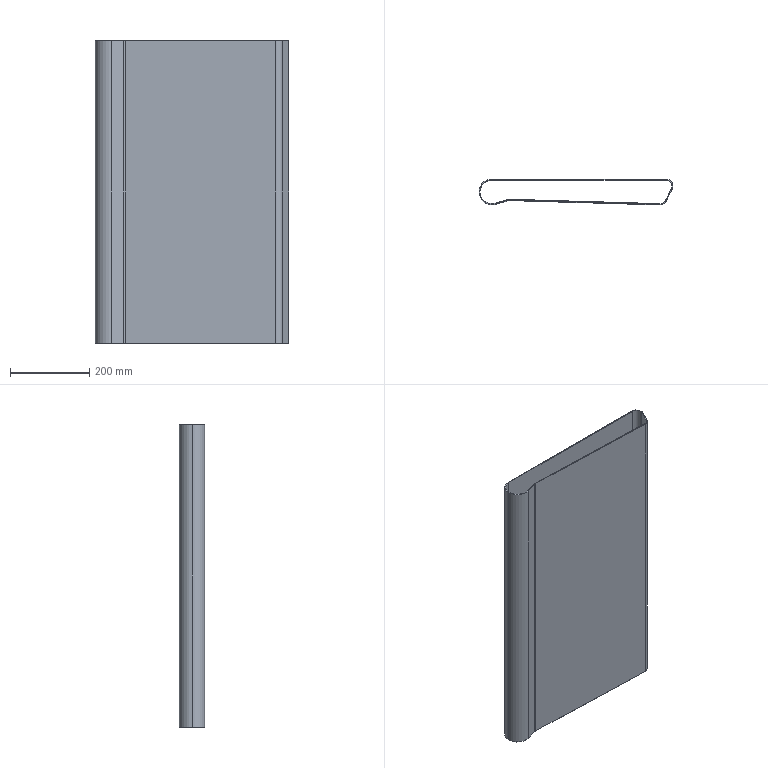Part | SolidWorks | features Extrusion 1 | 1 solid | 20 faces | box 489 x 64 x 765 mm | volume 1603169 mm3 | cylinder 10 | plane 10 | commonest cylinder face diameters 30 x2 34 x2 60 x2 64 x2 35 x1 39 x1
STEP:
#1=CARTESIAN_POINT('',(0.,30.,382.5));
#2=VERTEX_POINT('',#1);
#3=CARTESIAN_POINT('',(-30.,0.,382.5));
#4=VERTEX_POINT('',#3);
#5=CARTESIAN_POINT('',(0.,0.,382.5));
#6=DIRECTION('',(0.,0.,1.));
#7=DIRECTION('',(1.,0.,0.));
#8=AXIS2_PLACEMENT_3D('',#5,#6,#7);
#9=CIRCLE('',#8,30.);
#10=EDGE_CURVE('',#2,#4,#9,.T.);
#11=ORIENTED_EDGE('',*,*,#10,.T.);
#12=CARTESIAN_POINT('',(-30.,0.,-382.5));
#13=VERTEX_POINT('',#12);
#14=CARTESIAN_POINT('',(-30.,0.,382.5));
#15=DIRECTION('',(0.,0.,-1.));
#16=VECTOR('',#15,1000.);
#17=LINE('',#14,#16);
#18=EDGE_CURVE('',#4,#13,#17,.T.);
#19=ORIENTED_EDGE('',*,*,#18,.T.);
#20=CARTESIAN_POINT('',(0.,30.,-382.5));
#21=VERTEX_POINT('',#20);
#22=CARTESIAN_POINT('',(0.,0.,-382.5));
#23=DIRECTION('',(0.,0.,1.));
#24=DIRECTION('',(1.,0.,0.));
#25=AXIS2_PLACEMENT_3D('',#22,#23,#24);
#26=CIRCLE('',#25,30.);
#27=EDGE_CURVE('',#21,#13,#26,.T.);
#28=ORIENTED_EDGE('',*,*,#27,.F.);
#29=CARTESIAN_POINT('',(0.,30.,382.5));
#30=DIRECTION('',(0.,0.,-1.));
#31=VECTOR('',#30,1000.);
#32=LINE('',#29,#31);
#33=EDGE_CURVE('',#2,#21,#32,.T.);
#34=ORIENTED_EDGE('',*,*,#33,.F.);
#35=EDGE_LOOP('',(#11,#19,#28,#34));
#36=FACE_OUTER_BOUND('',#35,.T.);
#37=CARTESIAN_POINT('',(0.,0.,382.5));
#38=DIRECTION('',(0.,0.,-1.));
#39=DIRECTION('',(-1.,0.,0.));
#40=AXIS2_PLACEMENT_3D('',#37,#38,#39);
#41=CYLINDRICAL_SURFACE('',#40,30.);
#42=ADVANCED_FACE('',(#36),#41,.F.);
#43=CARTESIAN_POINT('',(-32.,0.,382.5));
#44=VERTEX_POINT('',#43);
#45=CARTESIAN_POINT('',(8.903,-30.737,382.5));
#46=VERTEX_POINT('',#45);
#47=CARTESIAN_POINT('',(0.,0.,382.5));
#48=DIRECTION('',(0.,0.,1.));
#49=DIRECTION('',(1.,0.,0.));
#50=AXIS2_PLACEMENT_3D('',#47,#48,#49);
#51=CIRCLE('',#50,32.);
#52=EDGE_CURVE('',#44,#46,#51,.T.);
#53=ORIENTED_EDGE('',*,*,#52,.F.);
#54=CARTESIAN_POINT('',(-32.,0.,-382.5));
#55=VERTEX_POINT('',#54);
#56=CARTESIAN_POINT('',(-32.,0.,382.5));
#57=DIRECTION('',(0.,0.,-1.));
#58=VECTOR('',#57,1000.);
#59=LINE('',#56,#58);
#60=EDGE_CURVE('',#44,#55,#59,.T.);
#61=ORIENTED_EDGE('',*,*,#60,.T.);
#62=CARTESIAN_POINT('',(8.903,-30.737,-382.5));
#63=VERTEX_POINT('',#62);
#64=CARTESIAN_POINT('',(0.,0.,-382.5));
#65=DIRECTION('',(0.,0.,1.));
#66=DIRECTION('',(1.,0.,0.));
#67=AXIS2_PLACEMENT_3D('',#64,#65,#66);
#68=CIRCLE('',#67,32.);
#69=EDGE_CURVE('',#55,#63,#68,.T.);
#70=ORIENTED_EDGE('',*,*,#69,.T.);
#71=CARTESIAN_POINT('',(8.903,-30.737,382.5));
#72=DIRECTION('',(0.,0.,-1.));
#73=VECTOR('',#72,1000.);
#74=LINE('',#71,#73);
#75=EDGE_CURVE('',#46,#63,#74,.T.);
#76=ORIENTED_EDGE('',*,*,#75,.F.);
#77=EDGE_LOOP('',(#53,#61,#70,#76));
#78=FACE_OUTER_BOUND('',#77,.T.);
#79=CARTESIAN_POINT('',(0.,0.,382.5));
#80=DIRECTION('',(0.,0.,-1.));
#81=DIRECTION('',(-1.,0.,0.));
#82=AXIS2_PLACEMENT_3D('',#79,#80,#81);
#83=CYLINDRICAL_SURFACE('',#82,32.);
#84=ADVANCED_FACE('',(#78),#83,.T.);
#85=CARTESIAN_POINT('',(0.,32.,382.5));
#86=VERTEX_POINT('',#85);
#87=CARTESIAN_POINT('',(0.,0.,382.5));
#88=DIRECTION('',(0.,0.,1.));
#89=DIRECTION('',(1.,0.,0.));
#90=AXIS2_PLACEMENT_3D('',#87,#88,#89);
#91=CIRCLE('',#90,32.);
#92=EDGE_CURVE('',#86,#44,#91,.T.);
#93=ORIENTED_EDGE('',*,*,#92,.T.);
#94=ORIENTED_EDGE('',*,*,#52,.T.);
#95=CARTESIAN_POINT('',(40.131,-21.691,382.5));
#96=VERTEX_POINT('',#95);
#97=CARTESIAN_POINT('',(8.903,-30.737,382.5));
#98=DIRECTION('',(0.9605,0.2782,0.));
#99=VECTOR('',#98,1000.);
#100=LINE('',#97,#99);
#101=EDGE_CURVE('',#46,#96,#100,.T.);
#102=ORIENTED_EDGE('',*,*,#101,.T.);
#103=CARTESIAN_POINT('',(45.507,-21.007,382.5));
#104=VERTEX_POINT('',#103);
#105=CARTESIAN_POINT('',(45.,-38.5,382.5));
#106=DIRECTION('',(0.,0.,-1.));
#107=DIRECTION('',(1.,0.,0.));
#108=AXIS2_PLACEMENT_3D('',#105,#106,#107);
#109=CIRCLE('',#108,17.5);
#110=EDGE_CURVE('',#96,#104,#109,.T.);
#111=ORIENTED_EDGE('',*,*,#110,.T.);
#112=CARTESIAN_POINT('',(424.507,-31.993,382.5));
#113=VERTEX_POINT('',#112);
#114=CARTESIAN_POINT('',(45.507,-21.007,382.5));
#115=DIRECTION('',(0.9996,-0.02897,0.));
#116=VECTOR('',#115,1000.);
#117=LINE('',#114,#116);
#118=EDGE_CURVE('',#104,#113,#117,.T.);
#119=ORIENTED_EDGE('',*,*,#118,.T.);
#120=CARTESIAN_POINT('',(440.205,-22.603,382.5));
#121=VERTEX_POINT('',#120);
#122=CARTESIAN_POINT('',(425.,-15.,382.5));
#123=DIRECTION('',(0.,0.,1.));
#124=DIRECTION('',(1.,0.,0.));
#125=AXIS2_PLACEMENT_3D('',#122,#123,#124);
#126=CIRCLE('',#125,17.);
#127=EDGE_CURVE('',#113,#121,#126,.T.);
#128=ORIENTED_EDGE('',*,*,#127,.T.);
#129=CARTESIAN_POINT('',(455.205,7.397,382.5));
#130=VERTEX_POINT('',#129);
#131=CARTESIAN_POINT('',(455.205,7.397,382.5));
#132=DIRECTION('',(0.4472,0.8944,0.));
#133=VECTOR('',#132,1000.);
#134=LINE('',#131,#133);
#135=EDGE_CURVE('',#121,#130,#134,.T.);
#136=ORIENTED_EDGE('',*,*,#135,.T.);
#137=CARTESIAN_POINT('',(440.,32.,382.5));
#138=VERTEX_POINT('',#137);
#139=CARTESIAN_POINT('',(440.,15.,382.5));
#140=DIRECTION('',(0.,0.,1.));
#141=DIRECTION('',(1.,0.,0.));
#142=AXIS2_PLACEMENT_3D('',#139,#140,#141);
#143=CIRCLE('',#142,17.);
#144=EDGE_CURVE('',#130,#138,#143,.T.);
#145=ORIENTED_EDGE('',*,*,#144,.T.);
#146=CARTESIAN_POINT('',(0.,32.,382.5));
#147=DIRECTION('',(-1.,0.,0.));
#148=VECTOR('',#147,1000.);
#149=LINE('',#146,#148);
#150=EDGE_CURVE('',#138,#86,#149,.T.);
#151=ORIENTED_EDGE('',*,*,#150,.T.);
#152=EDGE_LOOP('',(#93,#94,#102,#111,#119,#128,#136,#145,#151));
#153=FACE_OUTER_BOUND('',#152,.T.);
#154=CARTESIAN_POINT('',(8.347,-28.815,382.5));
#155=VERTEX_POINT('',#154);
#156=CARTESIAN_POINT('',(39.575,-19.77,382.5));
#157=VERTEX_POINT('',#156);
#158=CARTESIAN_POINT('',(8.347,-28.815,382.5));
#159=DIRECTION('',(0.9605,0.2782,0.));
#160=VECTOR('',#159,1000.);
#161=LINE('',#158,#160);
#162=EDGE_CURVE('',#155,#157,#161,.T.);
#163=ORIENTED_EDGE('',*,*,#162,.F.);
#164=CARTESIAN_POINT('',(0.,0.,382.5));
#165=DIRECTION('',(0.,0.,1.));
#166=DIRECTION('',(1.,0.,0.));
#167=AXIS2_PLACEMENT_3D('',#164,#165,#166);
#168=CIRCLE('',#167,30.);
#169=EDGE_CURVE('',#4,#155,#168,.T.);
#170=ORIENTED_EDGE('',*,*,#169,.F.);
#171=ORIENTED_EDGE('',*,*,#10,.F.);
#172=CARTESIAN_POINT('',(440.,30.,382.5));
#173=VERTEX_POINT('',#172);
#174=CARTESIAN_POINT('',(0.,30.,382.5));
#175=DIRECTION('',(-1.,0.,0.));
#176=VECTOR('',#175,1000.);
#177=LINE('',#174,#176);
#178=EDGE_CURVE('',#173,#2,#177,.T.);
#179=ORIENTED_EDGE('',*,*,#178,.F.);
#180=CARTESIAN_POINT('',(453.416,8.292,382.5));
#181=VERTEX_POINT('',#180);
#182=CARTESIAN_POINT('',(440.,15.,382.5));
#183=DIRECTION('',(0.,0.,1.));
#184=DIRECTION('',(1.,0.,0.));
#185=AXIS2_PLACEMENT_3D('',#182,#183,#184);
#186=CIRCLE('',#185,15.);
#187=EDGE_CURVE('',#181,#173,#186,.T.);
#188=ORIENTED_EDGE('',*,*,#187,.F.);
#189=CARTESIAN_POINT('',(438.416,-21.708,382.5));
#190=VERTEX_POINT('',#189);
#191=CARTESIAN_POINT('',(453.416,8.292,382.5));
#192=DIRECTION('',(0.4472,0.8944,0.));
#193=VECTOR('',#192,1000.);
#194=LINE('',#191,#193);
#195=EDGE_CURVE('',#190,#181,#194,.T.);
#196=ORIENTED_EDGE('',*,*,#195,.F.);
#197=CARTESIAN_POINT('',(424.565,-29.994,382.5));
#198=VERTEX_POINT('',#197);
#199=CARTESIAN_POINT('',(425.,-15.,382.5));
#200=DIRECTION('',(0.,0.,1.));
#201=DIRECTION('',(1.,0.,0.));
#202=AXIS2_PLACEMENT_3D('',#199,#200,#201);
#203=CIRCLE('',#202,15.);
#204=EDGE_CURVE('',#198,#190,#203,.T.);
#205=ORIENTED_EDGE('',*,*,#204,.F.);
#206=CARTESIAN_POINT('',(45.565,-19.008,382.5));
#207=VERTEX_POINT('',#206);
#208=CARTESIAN_POINT('',(45.565,-19.008,382.5));
#209=DIRECTION('',(0.9996,-0.02897,0.));
#210=VECTOR('',#209,1000.);
#211=LINE('',#208,#210);
#212=EDGE_CURVE('',#207,#198,#211,.T.);
#213=ORIENTED_EDGE('',*,*,#212,.F.);
#214=CARTESIAN_POINT('',(45.,-38.5,382.5));
#215=DIRECTION('',(0.,0.,-1.));
#216=DIRECTION('',(1.,0.,0.));
#217=AXIS2_PLACEMENT_3D('',#214,#215,#216);
#218=CIRCLE('',#217,19.5);
#219=EDGE_CURVE('',#157,#207,#218,.T.);
#220=ORIENTED_EDGE('',*,*,#219,.F.);
#221=EDGE_LOOP('',(#163,#170,#171,#179,#188,#196,#205,#213,#220));
#222=FACE_BOUND('',#221,.T.);
#223=CARTESIAN_POINT('',(0.,0.,382.5));
#224=DIRECTION('',(0.,0.,1.));
#225=DIRECTION('',(1.,0.,0.));
#226=AXIS2_PLACEMENT_3D('',#223,#224,#225);
#227=PLANE('',#226);
#228=ADVANCED_FACE('',(#153,#222),#227,.T.);
#229=CARTESIAN_POINT('',(0.,32.,-382.5));
#230=VERTEX_POINT('',#229);
#231=CARTESIAN_POINT('',(0.,0.,-382.5));
#232=DIRECTION('',(0.,0.,1.));
#233=DIRECTION('',(1.,0.,0.));
#234=AXIS2_PLACEMENT_3D('',#231,#232,#233);
#235=CIRCLE('',#234,32.);
#236=EDGE_CURVE('',#230,#55,#235,.T.);
#237=ORIENTED_EDGE('',*,*,#236,.F.);
#238=CARTESIAN_POINT('',(440.,32.,-382.5));
#239=VERTEX_POINT('',#238);
#240=CARTESIAN_POINT('',(0.,32.,-382.5));
#241=DIRECTION('',(-1.,0.,0.));
#242=VECTOR('',#241,1000.);
#243=LINE('',#240,#242);
#244=EDGE_CURVE('',#239,#230,#243,.T.);
#245=ORIENTED_EDGE('',*,*,#244,.F.);
#246=CARTESIAN_POINT('',(455.205,7.397,-382.5));
#247=VERTEX_POINT('',#246);
#248=CARTESIAN_POINT('',(440.,15.,-382.5));
#249=DIRECTION('',(0.,0.,1.));
#250=DIRECTION('',(1.,0.,0.));
#251=AXIS2_PLACEMENT_3D('',#248,#249,#250);
#252=CIRCLE('',#251,17.);
#253=EDGE_CURVE('',#247,#239,#252,.T.);
#254=ORIENTED_EDGE('',*,*,#253,.F.);
#255=CARTESIAN_POINT('',(440.205,-22.603,-382.5));
#256=VERTEX_POINT('',#255);
#257=CARTESIAN_POINT('',(455.205,7.397,-382.5));
#258=DIRECTION('',(0.4472,0.8944,0.));
#259=VECTOR('',#258,1000.);
#260=LINE('',#257,#259);
#261=EDGE_CURVE('',#256,#247,#260,.T.);
#262=ORIENTED_EDGE('',*,*,#261,.F.);
#263=CARTESIAN_POINT('',(424.507,-31.993,-382.5));
#264=VERTEX_POINT('',#263);
#265=CARTESIAN_POINT('',(425.,-15.,-382.5));
#266=DIRECTION('',(0.,0.,1.));
#267=DIRECTION('',(1.,0.,0.));
#268=AXIS2_PLACEMENT_3D('',#265,#266,#267);
#269=CIRCLE('',#268,17.);
#270=EDGE_CURVE('',#264,#256,#269,.T.);
#271=ORIENTED_EDGE('',*,*,#270,.F.);
#272=CARTESIAN_POINT('',(45.507,-21.007,-382.5));
#273=VERTEX_POINT('',#272);
#274=CARTESIAN_POINT('',(45.507,-21.007,-382.5));
#275=DIRECTION('',(0.9996,-0.02897,0.));
#276=VECTOR('',#275,1000.);
#277=LINE('',#274,#276);
#278=EDGE_CURVE('',#273,#264,#277,.T.);
#279=ORIENTED_EDGE('',*,*,#278,.F.);
#280=CARTESIAN_POINT('',(40.131,-21.691,-382.5));
#281=VERTEX_POINT('',#280);
#282=CARTESIAN_POINT('',(45.,-38.5,-382.5));
#283=DIRECTION('',(0.,0.,-1.));
#284=DIRECTION('',(1.,0.,0.));
#285=AXIS2_PLACEMENT_3D('',#282,#283,#284);
#286=CIRCLE('',#285,17.5);
#287=EDGE_CURVE('',#281,#273,#286,.T.);
#288=ORIENTED_EDGE('',*,*,#287,.F.);
#289=CARTESIAN_POINT('',(8.903,-30.737,-382.5));
#290=DIRECTION('',(0.9605,0.2782,0.));
#291=VECTOR('',#290,1000.);
#292=LINE('',#289,#291);
#293=EDGE_CURVE('',#63,#281,#292,.T.);
#294=ORIENTED_EDGE('',*,*,#293,.F.);
#295=ORIENTED_EDGE('',*,*,#69,.F.);
#296=EDGE_LOOP('',(#237,#245,#254,#262,#271,#279,#288,#294,#295));
#297=FACE_OUTER_BOUND('',#296,.T.);
#298=ORIENTED_EDGE('',*,*,#27,.T.);
#299=CARTESIAN_POINT('',(8.347,-28.815,-382.5));
#300=VERTEX_POINT('',#299);
#301=CARTESIAN_POINT('',(0.,0.,-382.5));
#302=DIRECTION('',(0.,0.,1.));
#303=DIRECTION('',(1.,0.,0.));
#304=AXIS2_PLACEMENT_3D('',#301,#302,#303);
#305=CIRCLE('',#304,30.);
#306=EDGE_CURVE('',#13,#300,#305,.T.);
#307=ORIENTED_EDGE('',*,*,#306,.T.);
#308=CARTESIAN_POINT('',(39.575,-19.77,-382.5));
#309=VERTEX_POINT('',#308);
#310=CARTESIAN_POINT('',(8.347,-28.815,-382.5));
#311=DIRECTION('',(0.9605,0.2782,0.));
#312=VECTOR('',#311,1000.);
#313=LINE('',#310,#312);
#314=EDGE_CURVE('',#300,#309,#313,.T.);
#315=ORIENTED_EDGE('',*,*,#314,.T.);
#316=CARTESIAN_POINT('',(45.565,-19.008,-382.5));
#317=VERTEX_POINT('',#316);
#318=CARTESIAN_POINT('',(45.,-38.5,-382.5));
#319=DIRECTION('',(0.,0.,-1.));
#320=DIRECTION('',(1.,0.,0.));
#321=AXIS2_PLACEMENT_3D('',#318,#319,#320);
#322=CIRCLE('',#321,19.5);
#323=EDGE_CURVE('',#309,#317,#322,.T.);
#324=ORIENTED_EDGE('',*,*,#323,.T.);
#325=CARTESIAN_POINT('',(424.565,-29.994,-382.5));
#326=VERTEX_POINT('',#325);
#327=CARTESIAN_POINT('',(45.565,-19.008,-382.5));
#328=DIRECTION('',(0.9996,-0.02897,0.));
#329=VECTOR('',#328,1000.);
#330=LINE('',#327,#329);
#331=EDGE_CURVE('',#317,#326,#330,.T.);
#332=ORIENTED_EDGE('',*,*,#331,.T.);
#333=CARTESIAN_POINT('',(438.416,-21.708,-382.5));
#334=VERTEX_POINT('',#333);
#335=CARTESIAN_POINT('',(425.,-15.,-382.5));
#336=DIRECTION('',(0.,0.,1.));
#337=DIRECTION('',(1.,0.,0.));
#338=AXIS2_PLACEMENT_3D('',#335,#336,#337);
#339=CIRCLE('',#338,15.);
#340=EDGE_CURVE('',#326,#334,#339,.T.);
#341=ORIENTED_EDGE('',*,*,#340,.T.);
#342=CARTESIAN_POINT('',(453.416,8.292,-382.5));
#343=VERTEX_POINT('',#342);
#344=CARTESIAN_POINT('',(453.416,8.292,-382.5));
#345=DIRECTION('',(0.4472,0.8944,0.));
#346=VECTOR('',#345,1000.);
#347=LINE('',#344,#346);
#348=EDGE_CURVE('',#334,#343,#347,.T.);
#349=ORIENTED_EDGE('',*,*,#348,.T.);
#350=CARTESIAN_POINT('',(440.,30.,-382.5));
#351=VERTEX_POINT('',#350);
#352=CARTESIAN_POINT('',(440.,15.,-382.5));
#353=DIRECTION('',(0.,0.,1.));
#354=DIRECTION('',(1.,0.,0.));
#355=AXIS2_PLACEMENT_3D('',#352,#353,#354);
#356=CIRCLE('',#355,15.);
#357=EDGE_CURVE('',#343,#351,#356,.T.);
#358=ORIENTED_EDGE('',*,*,#357,.T.);
#359=CARTESIAN_POINT('',(0.,30.,-382.5));
#360=DIRECTION('',(-1.,0.,0.));
#361=VECTOR('',#360,1000.);
#362=LINE('',#359,#361);
#363=EDGE_CURVE('',#351,#21,#362,.T.);
#364=ORIENTED_EDGE('',*,*,#363,.T.);
#365=EDGE_LOOP('',(#298,#307,#315,#324,#332,#341,#349,#358,#364));
#366=FACE_BOUND('',#365,.T.);
#367=CARTESIAN_POINT('',(0.,0.,-382.5));
#368=DIRECTION('',(0.,0.,1.));
#369=DIRECTION('',(1.,0.,0.));
#370=AXIS2_PLACEMENT_3D('',#367,#368,#369);
#371=PLANE('',#370);
#372=ADVANCED_FACE('',(#297,#366),#371,.F.);
#373=ORIENTED_EDGE('',*,*,#60,.F.);
#374=ORIENTED_EDGE('',*,*,#92,.F.);
#375=CARTESIAN_POINT('',(0.,32.,382.5));
#376=DIRECTION('',(0.,0.,-1.));
#377=VECTOR('',#376,1000.);
#378=LINE('',#375,#377);
#379=EDGE_CURVE('',#86,#230,#378,.T.);
#380=ORIENTED_EDGE('',*,*,#379,.T.);
#381=ORIENTED_EDGE('',*,*,#236,.T.);
#382=EDGE_LOOP('',(#373,#374,#380,#381));
#383=FACE_OUTER_BOUND('',#382,.T.);
#384=CARTESIAN_POINT('',(0.,0.,382.5));
#385=DIRECTION('',(0.,0.,-1.));
#386=DIRECTION('',(-1.,0.,0.));
#387=AXIS2_PLACEMENT_3D('',#384,#385,#386);
#388=CYLINDRICAL_SURFACE('',#387,32.);
#389=ADVANCED_FACE('',(#383),#388,.T.);
#390=ORIENTED_EDGE('',*,*,#293,.T.);
#391=CARTESIAN_POINT('',(40.131,-21.691,382.5));
#392=DIRECTION('',(0.,0.,-1.));
#393=VECTOR('',#392,1000.);
#394=LINE('',#391,#393);
#395=EDGE_CURVE('',#96,#281,#394,.T.);
#396=ORIENTED_EDGE('',*,*,#395,.F.);
#397=ORIENTED_EDGE('',*,*,#101,.F.);
#398=ORIENTED_EDGE('',*,*,#75,.T.);
#399=EDGE_LOOP('',(#390,#396,#397,#398));
#400=FACE_OUTER_BOUND('',#399,.T.);
#401=CARTESIAN_POINT('',(8.903,-30.737,382.5));
#402=DIRECTION('',(-0.2782,0.9605,0.));
#403=DIRECTION('',(-0.9605,-0.2782,0.));
#404=AXIS2_PLACEMENT_3D('',#401,#402,#403);
#405=PLANE('',#404);
#406=ADVANCED_FACE('',(#400),#405,.F.);
#407=ORIENTED_EDGE('',*,*,#287,.T.);
#408=CARTESIAN_POINT('',(45.507,-21.007,382.5));
#409=DIRECTION('',(0.,0.,-1.));
#410=VECTOR('',#409,1000.);
#411=LINE('',#408,#410);
#412=EDGE_CURVE('',#104,#273,#411,.T.);
#413=ORIENTED_EDGE('',*,*,#412,.F.);
#414=ORIENTED_EDGE('',*,*,#110,.F.);
#415=ORIENTED_EDGE('',*,*,#395,.T.);
#416=EDGE_LOOP('',(#407,#413,#414,#415));
#417=FACE_OUTER_BOUND('',#416,.T.);
#418=CARTESIAN_POINT('',(45.,-38.5,382.5));
#419=DIRECTION('',(0.,0.,-1.));
#420=DIRECTION('',(-1.,0.,0.));
#421=AXIS2_PLACEMENT_3D('',#418,#419,#420);
#422=CYLINDRICAL_SURFACE('',#421,17.5);
#423=ADVANCED_FACE('',(#417),#422,.F.);
#424=ORIENTED_EDGE('',*,*,#278,.T.);
#425=CARTESIAN_POINT('',(424.507,-31.993,382.5));
#426=DIRECTION('',(0.,0.,-1.));
#427=VECTOR('',#426,1000.);
#428=LINE('',#425,#427);
#429=EDGE_CURVE('',#113,#264,#428,.T.);
#430=ORIENTED_EDGE('',*,*,#429,.F.);
#431=ORIENTED_EDGE('',*,*,#118,.F.);
#432=ORIENTED_EDGE('',*,*,#412,.T.);
#433=EDGE_LOOP('',(#424,#430,#431,#432));
#434=FACE_OUTER_BOUND('',#433,.T.);
#435=CARTESIAN_POINT('',(45.507,-21.007,382.5));
#436=DIRECTION('',(0.02897,0.9996,0.));
#437=DIRECTION('',(-0.9996,0.02897,0.));
#438=AXIS2_PLACEMENT_3D('',#435,#436,#437);
#439=PLANE('',#438);
#440=ADVANCED_FACE('',(#434),#439,.F.);
#441=ORIENTED_EDGE('',*,*,#270,.T.);
#442=CARTESIAN_POINT('',(440.205,-22.603,382.5));
#443=DIRECTION('',(0.,0.,-1.));
#444=VECTOR('',#443,1000.);
#445=LINE('',#442,#444);
#446=EDGE_CURVE('',#121,#256,#445,.T.);
#447=ORIENTED_EDGE('',*,*,#446,.F.);
#448=ORIENTED_EDGE('',*,*,#127,.F.);
#449=ORIENTED_EDGE('',*,*,#429,.T.);
#450=EDGE_LOOP('',(#441,#447,#448,#449));
#451=FACE_OUTER_BOUND('',#450,.T.);
#452=CARTESIAN_POINT('',(425.,-15.,382.5));
#453=DIRECTION('',(0.,0.,-1.));
#454=DIRECTION('',(-1.,0.,0.));
#455=AXIS2_PLACEMENT_3D('',#452,#453,#454);
#456=CYLINDRICAL_SURFACE('',#455,17.);
#457=ADVANCED_FACE('',(#451),#456,.T.);
#458=ORIENTED_EDGE('',*,*,#261,.T.);
#459=CARTESIAN_POINT('',(455.205,7.397,382.5));
#460=DIRECTION('',(0.,0.,-1.));
#461=VECTOR('',#460,1000.);
#462=LINE('',#459,#461);
#463=EDGE_CURVE('',#130,#247,#462,.T.);
#464=ORIENTED_EDGE('',*,*,#463,.F.);
#465=ORIENTED_EDGE('',*,*,#135,.F.);
#466=ORIENTED_EDGE('',*,*,#446,.T.);
#467=EDGE_LOOP('',(#458,#464,#465,#466));
#468=FACE_OUTER_BOUND('',#467,.T.);
#469=CARTESIAN_POINT('',(455.205,7.397,382.5));
#470=DIRECTION('',(-0.8944,0.4472,0.));
#471=DIRECTION('',(-0.4472,-0.8944,0.));
#472=AXIS2_PLACEMENT_3D('',#469,#470,#471);
#473=PLANE('',#472);
#474=ADVANCED_FACE('',(#468),#473,.F.);
#475=ORIENTED_EDGE('',*,*,#253,.T.);
#476=CARTESIAN_POINT('',(440.,32.,382.5));
#477=DIRECTION('',(0.,0.,-1.));
#478=VECTOR('',#477,1000.);
#479=LINE('',#476,#478);
#480=EDGE_CURVE('',#138,#239,#479,.T.);
#481=ORIENTED_EDGE('',*,*,#480,.F.);
#482=ORIENTED_EDGE('',*,*,#144,.F.);
#483=ORIENTED_EDGE('',*,*,#463,.T.);
#484=EDGE_LOOP('',(#475,#481,#482,#483));
#485=FACE_OUTER_BOUND('',#484,.T.);
#486=CARTESIAN_POINT('',(440.,15.,382.5));
#487=DIRECTION('',(0.,0.,-1.));
#488=DIRECTION('',(-1.,0.,0.));
#489=AXIS2_PLACEMENT_3D('',#486,#487,#488);
#490=CYLINDRICAL_SURFACE('',#489,17.);
#491=ADVANCED_FACE('',(#485),#490,.T.);
#492=ORIENTED_EDGE('',*,*,#244,.T.);
#493=ORIENTED_EDGE('',*,*,#379,.F.);
#494=ORIENTED_EDGE('',*,*,#150,.F.);
#495=ORIENTED_EDGE('',*,*,#480,.T.);
#496=EDGE_LOOP('',(#492,#493,#494,#495));
#497=FACE_OUTER_BOUND('',#496,.T.);
#498=CARTESIAN_POINT('',(0.,32.,382.5));
#499=DIRECTION('',(0.,-1.,0.));
#500=DIRECTION('',(1.,0.,0.));
#501=AXIS2_PLACEMENT_3D('',#498,#499,#500);
#502=PLANE('',#501);
#503=ADVANCED_FACE('',(#497),#502,.F.);
#504=ORIENTED_EDGE('',*,*,#18,.F.);
#505=ORIENTED_EDGE('',*,*,#169,.T.);
#506=CARTESIAN_POINT('',(8.347,-28.815,382.5));
#507=DIRECTION('',(0.,0.,-1.));
#508=VECTOR('',#507,1000.);
#509=LINE('',#506,#508);
#510=EDGE_CURVE('',#155,#300,#509,.T.);
#511=ORIENTED_EDGE('',*,*,#510,.T.);
#512=ORIENTED_EDGE('',*,*,#306,.F.);
#513=EDGE_LOOP('',(#504,#505,#511,#512));
#514=FACE_OUTER_BOUND('',#513,.T.);
#515=CARTESIAN_POINT('',(0.,0.,382.5));
#516=DIRECTION('',(0.,0.,-1.));
#517=DIRECTION('',(-1.,0.,0.));
#518=AXIS2_PLACEMENT_3D('',#515,#516,#517);
#519=CYLINDRICAL_SURFACE('',#518,30.);
#520=ADVANCED_FACE('',(#514),#519,.F.);
#521=ORIENTED_EDGE('',*,*,#314,.F.);
#522=ORIENTED_EDGE('',*,*,#510,.F.);
#523=ORIENTED_EDGE('',*,*,#162,.T.);
#524=CARTESIAN_POINT('',(39.575,-19.77,382.5));
#525=DIRECTION('',(0.,0.,-1.));
#526=VECTOR('',#525,1000.);
#527=LINE('',#524,#526);
#528=EDGE_CURVE('',#157,#309,#527,.T.);
#529=ORIENTED_EDGE('',*,*,#528,.T.);
#530=EDGE_LOOP('',(#521,#522,#523,#529));
#531=FACE_OUTER_BOUND('',#530,.T.);
#532=CARTESIAN_POINT('',(8.347,-28.815,382.5));
#533=DIRECTION('',(-0.2782,0.9605,0.));
#534=DIRECTION('',(-0.9605,-0.2782,0.));
#535=AXIS2_PLACEMENT_3D('',#532,#533,#534);
#536=PLANE('',#535);
#537=ADVANCED_FACE('',(#531),#536,.T.);
#538=ORIENTED_EDGE('',*,*,#323,.F.);
#539=ORIENTED_EDGE('',*,*,#528,.F.);
#540=ORIENTED_EDGE('',*,*,#219,.T.);
#541=CARTESIAN_POINT('',(45.565,-19.008,382.5));
#542=DIRECTION('',(0.,0.,-1.));
#543=VECTOR('',#542,1000.);
#544=LINE('',#541,#543);
#545=EDGE_CURVE('',#207,#317,#544,.T.);
#546=ORIENTED_EDGE('',*,*,#545,.T.);
#547=EDGE_LOOP('',(#538,#539,#540,#546));
#548=FACE_OUTER_BOUND('',#547,.T.);
#549=CARTESIAN_POINT('',(45.,-38.5,382.5));
#550=DIRECTION('',(0.,0.,-1.));
#551=DIRECTION('',(-1.,0.,0.));
#552=AXIS2_PLACEMENT_3D('',#549,#550,#551);
#553=CYLINDRICAL_SURFACE('',#552,19.5);
#554=ADVANCED_FACE('',(#548),#553,.T.);
#555=ORIENTED_EDGE('',*,*,#331,.F.);
#556=ORIENTED_EDGE('',*,*,#545,.F.);
#557=ORIENTED_EDGE('',*,*,#212,.T.);
#558=CARTESIAN_POINT('',(424.565,-29.994,382.5));
#559=DIRECTION('',(0.,0.,-1.));
#560=VECTOR('',#559,1000.);
#561=LINE('',#558,#560);
#562=EDGE_CURVE('',#198,#326,#561,.T.);
#563=ORIENTED_EDGE('',*,*,#562,.T.);
#564=EDGE_LOOP('',(#555,#556,#557,#563));
#565=FACE_OUTER_BOUND('',#564,.T.);
#566=CARTESIAN_POINT('',(45.565,-19.008,382.5));
#567=DIRECTION('',(0.02897,0.9996,0.));
#568=DIRECTION('',(-0.9996,0.02897,0.));
#569=AXIS2_PLACEMENT_3D('',#566,#567,#568);
#570=PLANE('',#569);
#571=ADVANCED_FACE('',(#565),#570,.T.);
#572=ORIENTED_EDGE('',*,*,#340,.F.);
#573=ORIENTED_EDGE('',*,*,#562,.F.);
#574=ORIENTED_EDGE('',*,*,#204,.T.);
#575=CARTESIAN_POINT('',(438.416,-21.708,382.5));
#576=DIRECTION('',(0.,0.,-1.));
#577=VECTOR('',#576,1000.);
#578=LINE('',#575,#577);
#579=EDGE_CURVE('',#190,#334,#578,.T.);
#580=ORIENTED_EDGE('',*,*,#579,.T.);
#581=EDGE_LOOP('',(#572,#573,#574,#580));
#582=FACE_OUTER_BOUND('',#581,.T.);
#583=CARTESIAN_POINT('',(425.,-15.,382.5));
#584=DIRECTION('',(0.,0.,-1.));
#585=DIRECTION('',(-1.,0.,0.));
#586=AXIS2_PLACEMENT_3D('',#583,#584,#585);
#587=CYLINDRICAL_SURFACE('',#586,15.);
#588=ADVANCED_FACE('',(#582),#587,.F.);
#589=ORIENTED_EDGE('',*,*,#348,.F.);
#590=ORIENTED_EDGE('',*,*,#579,.F.);
#591=ORIENTED_EDGE('',*,*,#195,.T.);
#592=CARTESIAN_POINT('',(453.416,8.292,382.5));
#593=DIRECTION('',(0.,0.,-1.));
#594=VECTOR('',#593,1000.);
#595=LINE('',#592,#594);
#596=EDGE_CURVE('',#181,#343,#595,.T.);
#597=ORIENTED_EDGE('',*,*,#596,.T.);
#598=EDGE_LOOP('',(#589,#590,#591,#597));
#599=FACE_OUTER_BOUND('',#598,.T.);
#600=CARTESIAN_POINT('',(453.416,8.292,382.5));
#601=DIRECTION('',(-0.8944,0.4472,0.));
#602=DIRECTION('',(-0.4472,-0.8944,0.));
#603=AXIS2_PLACEMENT_3D('',#600,#601,#602);
#604=PLANE('',#603);
#605=ADVANCED_FACE('',(#599),#604,.T.);
#606=ORIENTED_EDGE('',*,*,#357,.F.);
#607=ORIENTED_EDGE('',*,*,#596,.F.);
#608=ORIENTED_EDGE('',*,*,#187,.T.);
#609=CARTESIAN_POINT('',(440.,30.,382.5));
#610=DIRECTION('',(0.,0.,-1.));
#611=VECTOR('',#610,1000.);
#612=LINE('',#609,#611);
#613=EDGE_CURVE('',#173,#351,#612,.T.);
#614=ORIENTED_EDGE('',*,*,#613,.T.);
#615=EDGE_LOOP('',(#606,#607,#608,#614));
#616=FACE_OUTER_BOUND('',#615,.T.);
#617=CARTESIAN_POINT('',(440.,15.,382.5));
#618=DIRECTION('',(0.,0.,-1.));
#619=DIRECTION('',(-1.,0.,0.));
#620=AXIS2_PLACEMENT_3D('',#617,#618,#619);
#621=CYLINDRICAL_SURFACE('',#620,15.);
#622=ADVANCED_FACE('',(#616),#621,.F.);
#623=ORIENTED_EDGE('',*,*,#363,.F.);
#624=ORIENTED_EDGE('',*,*,#613,.F.);
#625=ORIENTED_EDGE('',*,*,#178,.T.);
#626=ORIENTED_EDGE('',*,*,#33,.T.);
#627=EDGE_LOOP('',(#623,#624,#625,#626));
#628=FACE_OUTER_BOUND('',#627,.T.);
#629=CARTESIAN_POINT('',(0.,30.,382.5));
#630=DIRECTION('',(0.,-1.,0.));
#631=DIRECTION('',(1.,0.,0.));
#632=AXIS2_PLACEMENT_3D('',#629,#630,#631);
#633=PLANE('',#632);
#634=ADVANCED_FACE('',(#628),#633,.T.);
#635=CLOSED_SHELL('',(#42,#84,#228,#372,#389,#406,#423,#440,#457,#474,#491,#503,#520,#537,#554,#571,#588,#605,#622,#634));
#636=MANIFOLD_SOLID_BREP('',#635);
#637=CARTESIAN_POINT('',(0.,0.,0.));
#638=DIRECTION('',(0.,0.,1.));
#639=DIRECTION('',(1.,0.,0.));
#640=AXIS2_PLACEMENT_3D('',#637,#638,#639);
#641=(LENGTH_UNIT()NAMED_UNIT(*)SI_UNIT(.MILLI.,.METRE.));
#642=UNCERTAINTY_MEASURE_WITH_UNIT(LENGTH_MEASURE(0.00001),#641,'','');
#643=(NAMED_UNIT(*)PLANE_ANGLE_UNIT()SI_UNIT($,.RADIAN.));
#644=(NAMED_UNIT(*)SI_UNIT($,.STERADIAN.)SOLID_ANGLE_UNIT());
#645=(GEOMETRIC_REPRESENTATION_CONTEXT(3)GLOBAL_UNCERTAINTY_ASSIGNED_CONTEXT((#642))GLOBAL_UNIT_ASSIGNED_CONTEXT((#641,#643,#644))REPRESENTATION_CONTEXT('',''));
#646=ADVANCED_BREP_SHAPE_REPRESENTATION('',(#636,#640),#645);